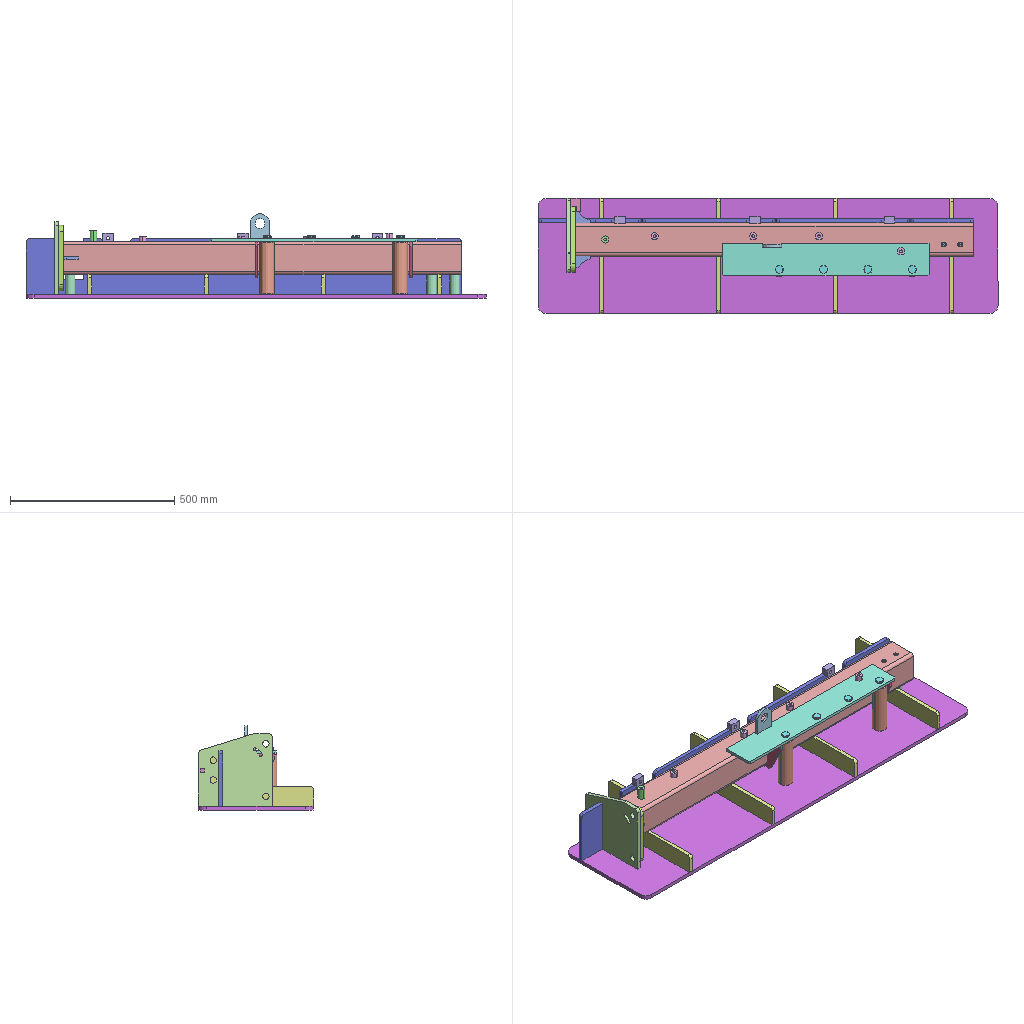Assembly | SolidWorks | 21 different items | 38 placed | box 1400 x 350 x 257 mm
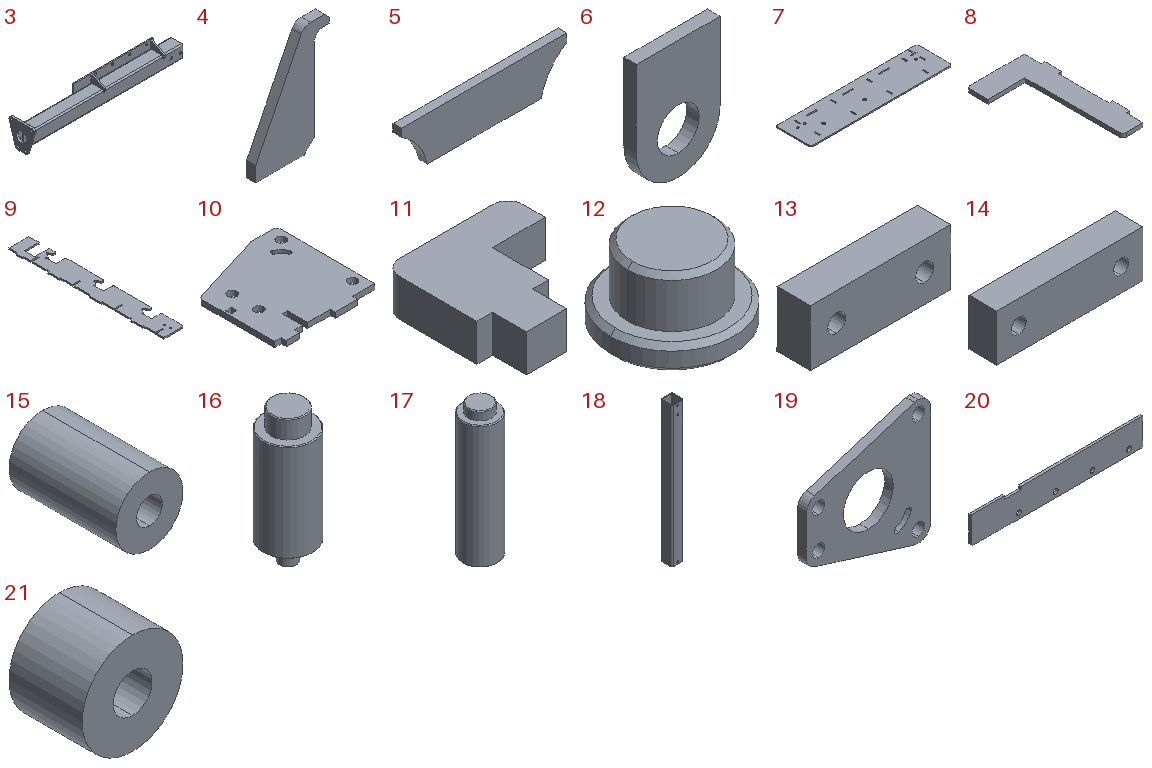Parts list (item | name | quantity | parent item | size | volume | features):
1 | 428-54-44441 Assembly Fixture Screw Seat Locating Plate1 | x1 | - | - | - | -
2 | 428-54-44441 Assembly Fixture Screw Seat Locating Plate2 | x1 | - | - | - | -
3 | (subassembly) | x1 | - | 1225 x 234.861 x 211 mm | 3400829 mm3 | features ReferencePattern 3, LocalLPattern 2
4 | - | x2 | in 3 | 72.5 x 9 x 110 mm | 37505 mm3 | features FlatPattern 1, SMBaseFlange 1, SheetMetal 1
5 | - | x1 | in 3 | 170 x 9 x 45 mm | 57559 mm3 | features FlatPattern 1, SMBaseFlange 1, SheetMetal 1
6 | - | x1 | in 3 | 60 x 9 x 85 mm | 36062 mm3 | features FlatPattern 1, SMBaseFlange 1, SheetMetal 1
7 | - | x1 | - | 1400 x 350 x 12 mm | 5725768 mm3 | features Fillet 1, FlatPattern 1, SMBaseFlange 1, SheetMetal 1
8 | - | x4 | - | 180 x 350 x 12 mm | 345781 mm3 | features Fillet 1, FlatPattern 1, SMBaseFlange 1, SheetMetal 1
9 | - | x1 | - | 180 x 1325 x 12 mm | 2282153 mm3 | features Fillet 2, FlatPattern 1, SMBaseFlange 1, SheetMetal 1
10 | - | x1 | - | 225 x 231 x 12 mm | 524877 mm3 | features Fillet 1, FlatPattern 1, SMBaseFlange 1, SheetMetal 1
11 | - | x1 | - | 40 x 41 x 12 mm | 12315 mm3 | features Fillet 1, FlatPattern 1, SMBaseFlange 1, SheetMetal 1
12 | - | x4 | - | 25 x 25 x 15 mm | 4924 mm3 | features Chamfer 1, Revolution 1
13 | - | x2 | in 3 | 80 x 19 x 32 mm | 45535 mm3 | features FlatPattern 1, HoleWzd 1, SMBaseFlange 1, SheetMetal 1
14 | - | x4 | in 3 | 100 x 19 x 32 mm | 57695 mm3 | features FlatPattern 1, HoleWzd 1, SMBaseFlange 1, SheetMetal 1
15 | - | x1 | in 3 | 22 x 35 x 22 mm | 11319 mm3 | features Extrusion 1, HoleWzd 1
16 | - | x3 | - | 30 x 30 x 81.5 mm | 46379 mm3 | features Chamfer 1, Revolution 1
17 | - | x2 | - | 45 x 45 x 178 mm | 262477 mm3 | features Chamfer 1, Revolution 1
18 | - | x1 | in 3 | 100 x 100 x 1211 mm | 1999990 mm3 | features ICE 4, Attribute 1, Extrusion 1
19 | - | x1 | in 3 | 200 x 14 x 199.722 mm | 327210 mm3 | features FlatPattern 1, SMBaseFlange 1, SheetMetal 1
20 | - | x1 | in 3 | 630 x 9 x 100 mm | 551134 mm3 | features FlatPattern 1, SMBaseFlange 1, SheetMetal 1
21 | - | x4 | in 3 | 22 x 16 x 22 mm | 5174 mm3 | features Extrusion 1, HoleWzd 1
Mates (type | each side: item.copy, entity, surface, feature):
In the top assembly
InPlace | 8.1 plane | assembly plane
InPlace | 8.2 face plane Base-Flange1 | 7.1 plane
Coincident | 7.1 face plane Base-Flange1 | 16.1 face plane Revolve1
Concentric | 18.1 face cylinder Cut-Extrude2 | 16.1 face cylinder Revolve1
Parallel | 19.1 face plane Base-Flange1 | 16.1 plane
Coincident | 7.1 face plane Base-Flange1 | 16.2 face plane Revolve1
Concentric | 18.1 face cylinder Cut-Extrude2 | 16.2 face cylinder Revolve1
Parallel | 8.1 face plane Base-Flange1 | 16.2 plane
Coincident | 7.1 face plane Base-Flange1 | 16.3 face plane Revolve1
Concentric | 18.1 face cylinder Cut-Extrude2 | 16.3 face cylinder Revolve1
Parallel | 8.1 face plane Base-Flange1 | 16.3 plane
Coincident | 7.1 face plane Base-Flange1 | 17.1 face plane Revolve1
Concentric | 20.1 face cylinder Base-Flange1 | 17.1 face cylinder Revolve1
Parallel | 8.3 face plane Base-Flange1 | 17.1 plane
Coincident | 7.1 face plane Base-Flange1 | 17.2 face plane Revolve1
Concentric | 20.1 face cylinder Base-Flange1 | 17.2 face cylinder Revolve1
Parallel | 18.1 face plane Boss-Extrude1 | 17.2 plane
InPlace | 8.2 face plane Base-Flange1 | 9.1 plane
InPlace | 3.1 face plane Base-Flange1 | 10.1 plane
InPlace | 3.1 face plane Base-Flange1 | 11.1 plane
In subassembly 3
Coincident | 18.2 face plane Cut-Extrude4 | 5.1 face plane Base-Flange1 | 2 times
DistanceDim | 18.2 face plane Boss-Extrude1 | 5.1 face plane Base-Flange1
Coincident | 18.2 face plane Boss-Extrude1 | 19.2 face plane Base-Flange1
DistanceDim | 19.2 face cylinder Base-Flange1 | 18.2 face plane Boss-Extrude1
DistanceDim | 18.2 face plane Boss-Extrude1 | 19.2 face cylinder Base-Flange1
Parallel | 18.2 face plane Boss-Extrude1 | 19.2 face plane Base-Flange1
Coincident | 18.2 face plane Boss-Extrude1 | 21.1 face plane Boss-Extrude1
DistanceDim | 19.2 face plane Base-Flange1 | 21.1 face cylinder Boss-Extrude1
DistanceDim | 18.2 face plane Boss-Extrude1 | 21.1 face cylinder Boss-Extrude1
Coincident | 18.2 face plane Boss-Extrude1 | 21.2 face plane Boss-Extrude1
DistanceDim | 18.2 face plane Boss-Extrude1 | 21.2 face cylinder Boss-Extrude1
DistanceDim | 21.2 face cylinder Boss-Extrude1 | 21.1 face cylinder Boss-Extrude1
Coincident | 18.2 face plane Boss-Extrude1 | 21.3 face plane Boss-Extrude1
DistanceDim | 18.2 face plane Boss-Extrude1 | 21.3 face cylinder Boss-Extrude1
DistanceDim | 21.3 face cylinder Boss-Extrude1 | 21.1 face cylinder Boss-Extrude1
Coincident | 18.2 face plane Boss-Extrude1 | 20.2 face plane Base-Flange1
DistanceDim | 19.2 face plane Base-Flange1 | 20.2 face plane Base-Flange1
DistanceDim | 18.2 face plane Boss-Extrude1 | 20.2 face plane Base-Flange1
Coincident | 20.2 face plane Base-Flange1 | 21.4 face plane Boss-Extrude1
DistanceDim | 18.2 face plane Boss-Extrude1 | 21.4 face cylinder Boss-Extrude1
DistanceDim | 19.2 face plane Base-Flange1 | 21.4 face cylinder Boss-Extrude1
Coincident | 18.2 face plane Boss-Extrude1 | 13.1 face plane Base-Flange1
Concentric | 18.2 face cylinder Cut-Extrude3 | 13.1 face cylinder M12 Tapped Hole1 | 2 times
Coincident | 18.2 face plane Boss-Extrude1 | 13.2 face plane Base-Flange1
Concentric | 18.2 face cylinder Cut-Extrude1 | 13.2 face cylinder M12 Tapped Hole1 | 2 times
Coincident | 18.2 face plane Boss-Extrude1 | 14.1 face plane Base-Flange1
Concentric | 18.2 face cylinder Cut-Extrude2 | 14.1 face cylinder M12 Tapped Hole1 | 2 times
Coincident | 18.2 face plane Boss-Extrude1 | 14.2 face plane Base-Flange1
DistanceDim | 19.2 face plane Base-Flange1 | 14.2 face plane Base-Flange1
DistanceDim | 18.2 face plane Boss-Extrude1 | 14.2 face cylinder M12 Tapped Hole1
Coincident | 18.2 face plane Boss-Extrude1 | 15.1 face plane Boss-Extrude1
DistanceDim | 15.1 face cylinder Boss-Extrude1 | 19.2 face plane Base-Flange1
DistanceDim | 18.2 face plane Boss-Extrude1 | 15.1 face cylinder Boss-Extrude1
Coincident | 18.2 face plane Boss-Extrude1 | 4.1 face plane Base-Flange1
Coincident | 20.2 face plane Base-Flange1 | 4.1 face plane Base-Flange1
DistanceDim | 20.2 face cylinder Base-Flange1 | 4.1 face plane Base-Flange1
Coincident | 18.2 face plane Boss-Extrude1 | 6.1 face plane Base-Flange1
Coincident | 20.2 face plane Base-Flange1 | 6.1 face plane Base-Flange1 | 2 times